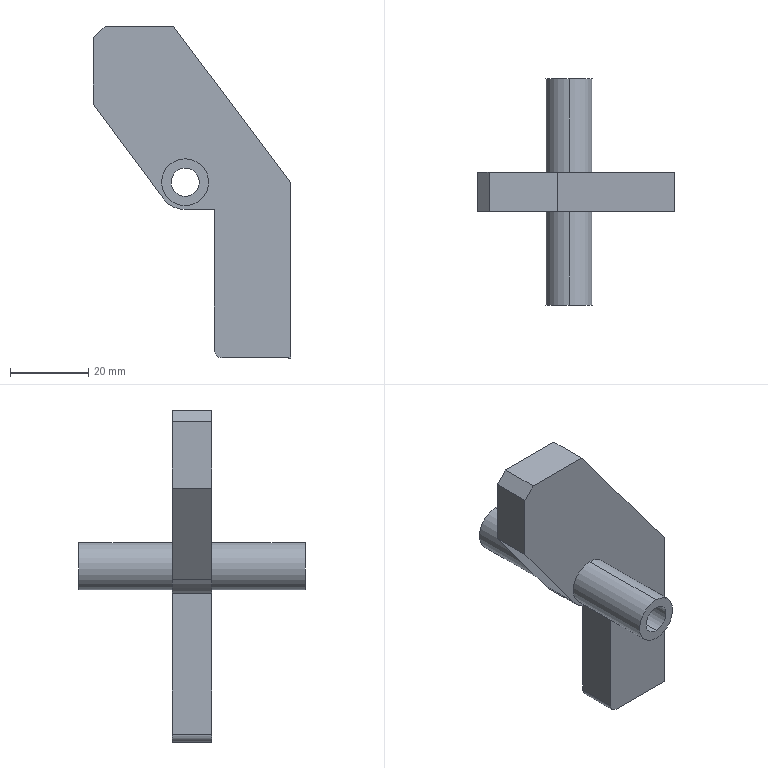Part | SolidWorks | features BaseBody 1 | 1 solid | 21 faces | box 50.5 x 58 x 85 mm | volume 25435 mm3 | plane 13 | cylinder 8 | commonest cylinder face diameters 12 x4 7.2 x2 4 x1 14 x1
STEP:
#1=CARTESIAN_POINT('',(896.946,-3871.973,948.971));
#2=VERTEX_POINT('',#1);
#3=CARTESIAN_POINT('',(896.946,-3871.973,960.971));
#4=VERTEX_POINT('',#3);
#5=CARTESIAN_POINT('',(896.946,-3871.973,954.971));
#6=DIRECTION('',(0.,-1.,0.));
#7=DIRECTION('',(0.,0.,-1.));
#8=AXIS2_PLACEMENT_3D('',#5,#6,#7);
#9=CIRCLE('',#8,6.);
#10=EDGE_CURVE('',#2,#4,#9,.T.);
#11=ORIENTED_EDGE('',*,*,#10,.T.);
#12=CARTESIAN_POINT('',(896.946,-3895.973,960.971));
#13=VERTEX_POINT('',#12);
#14=CARTESIAN_POINT('',(896.946,-3883.973,960.971));
#15=DIRECTION('',(0.,-1.,0.));
#16=VECTOR('',#15,1000.);
#17=LINE('',#14,#16);
#18=EDGE_CURVE('',#4,#13,#17,.T.);
#19=ORIENTED_EDGE('',*,*,#18,.T.);
#20=CARTESIAN_POINT('',(896.946,-3895.973,948.971));
#21=VERTEX_POINT('',#20);
#22=CARTESIAN_POINT('',(896.946,-3895.973,954.971));
#23=DIRECTION('',(0.,-1.,0.));
#24=DIRECTION('',(0.,0.,-1.));
#25=AXIS2_PLACEMENT_3D('',#22,#23,#24);
#26=CIRCLE('',#25,6.);
#27=EDGE_CURVE('',#21,#13,#26,.T.);
#28=ORIENTED_EDGE('',*,*,#27,.F.);
#29=CARTESIAN_POINT('',(896.946,-3883.973,948.971));
#30=DIRECTION('',(0.,-1.,0.));
#31=VECTOR('',#30,1000.);
#32=LINE('',#29,#31);
#33=EDGE_CURVE('',#2,#21,#32,.T.);
#34=ORIENTED_EDGE('',*,*,#33,.F.);
#35=EDGE_LOOP('',(#11,#19,#28,#34));
#36=FACE_OUTER_BOUND('',#35,.T.);
#37=CARTESIAN_POINT('',(896.946,-3883.973,954.971));
#38=DIRECTION('',(0.,-1.,0.));
#39=DIRECTION('',(0.,0.,-1.));
#40=AXIS2_PLACEMENT_3D('',#37,#38,#39);
#41=CYLINDRICAL_SURFACE('',#40,6.);
#42=ADVANCED_FACE('',(#36),#41,.T.);
#43=CARTESIAN_POINT('',(896.946,-3871.973,958.571));
#44=VERTEX_POINT('',#43);
#45=CARTESIAN_POINT('',(896.946,-3871.973,951.371));
#46=VERTEX_POINT('',#45);
#47=CARTESIAN_POINT('',(896.946,-3871.973,954.971));
#48=DIRECTION('',(0.,-1.,0.));
#49=DIRECTION('',(0.,0.,-1.));
#50=AXIS2_PLACEMENT_3D('',#47,#48,#49);
#51=CIRCLE('',#50,3.6);
#52=EDGE_CURVE('',#44,#46,#51,.T.);
#53=ORIENTED_EDGE('',*,*,#52,.F.);
#54=CARTESIAN_POINT('',(896.946,-3929.973,958.571));
#55=VERTEX_POINT('',#54);
#56=CARTESIAN_POINT('',(896.946,-3859.114,958.571));
#57=DIRECTION('',(0.,-1.,0.));
#58=VECTOR('',#57,1000.);
#59=LINE('',#56,#58);
#60=EDGE_CURVE('',#44,#55,#59,.T.);
#61=ORIENTED_EDGE('',*,*,#60,.T.);
#62=CARTESIAN_POINT('',(896.946,-3929.973,951.371));
#63=VERTEX_POINT('',#62);
#64=CARTESIAN_POINT('',(896.946,-3929.973,954.971));
#65=DIRECTION('',(0.,1.,0.));
#66=DIRECTION('',(0.,0.,-1.));
#67=AXIS2_PLACEMENT_3D('',#64,#65,#66);
#68=CIRCLE('',#67,3.6);
#69=EDGE_CURVE('',#63,#55,#68,.T.);
#70=ORIENTED_EDGE('',*,*,#69,.F.);
#71=CARTESIAN_POINT('',(896.946,-3859.114,951.371));
#72=DIRECTION('',(0.,-1.,0.));
#73=VECTOR('',#72,1000.);
#74=LINE('',#71,#73);
#75=EDGE_CURVE('',#46,#63,#74,.T.);
#76=ORIENTED_EDGE('',*,*,#75,.F.);
#77=EDGE_LOOP('',(#53,#61,#70,#76));
#78=FACE_OUTER_BOUND('',#77,.T.);
#79=CARTESIAN_POINT('',(896.946,-3859.114,954.971));
#80=DIRECTION('',(0.,-1.,0.));
#81=DIRECTION('',(0.,0.,-1.));
#82=AXIS2_PLACEMENT_3D('',#79,#80,#81);
#83=CYLINDRICAL_SURFACE('',#82,3.6);
#84=ADVANCED_FACE('',(#78),#83,.F.);
#85=CARTESIAN_POINT('',(896.946,-3905.973,948.971));
#86=VERTEX_POINT('',#85);
#87=CARTESIAN_POINT('',(896.946,-3905.973,960.971));
#88=VERTEX_POINT('',#87);
#89=CARTESIAN_POINT('',(896.946,-3905.973,954.971));
#90=DIRECTION('',(0.,-1.,0.));
#91=DIRECTION('',(0.,0.,-1.));
#92=AXIS2_PLACEMENT_3D('',#89,#90,#91);
#93=CIRCLE('',#92,6.);
#94=EDGE_CURVE('',#86,#88,#93,.T.);
#95=ORIENTED_EDGE('',*,*,#94,.T.);
#96=CARTESIAN_POINT('',(896.946,-3929.973,960.971));
#97=VERTEX_POINT('',#96);
#98=CARTESIAN_POINT('',(896.946,-3917.973,960.971));
#99=DIRECTION('',(0.,-1.,0.));
#100=VECTOR('',#99,1000.);
#101=LINE('',#98,#100);
#102=EDGE_CURVE('',#88,#97,#101,.T.);
#103=ORIENTED_EDGE('',*,*,#102,.T.);
#104=CARTESIAN_POINT('',(896.946,-3929.973,948.971));
#105=VERTEX_POINT('',#104);
#106=CARTESIAN_POINT('',(896.946,-3929.973,954.971));
#107=DIRECTION('',(0.,1.,0.));
#108=DIRECTION('',(0.,0.,-1.));
#109=AXIS2_PLACEMENT_3D('',#106,#107,#108);
#110=CIRCLE('',#109,6.);
#111=EDGE_CURVE('',#97,#105,#110,.T.);
#112=ORIENTED_EDGE('',*,*,#111,.T.);
#113=CARTESIAN_POINT('',(896.946,-3917.973,948.971));
#114=DIRECTION('',(0.,-1.,0.));
#115=VECTOR('',#114,1000.);
#116=LINE('',#113,#115);
#117=EDGE_CURVE('',#86,#105,#116,.T.);
#118=ORIENTED_EDGE('',*,*,#117,.F.);
#119=EDGE_LOOP('',(#95,#103,#112,#118));
#120=FACE_OUTER_BOUND('',#119,.T.);
#121=CARTESIAN_POINT('',(896.946,-3917.973,954.971));
#122=DIRECTION('',(0.,-1.,0.));
#123=DIRECTION('',(0.,0.,-1.));
#124=AXIS2_PLACEMENT_3D('',#121,#122,#123);
#125=CYLINDRICAL_SURFACE('',#124,6.);
#126=ADVANCED_FACE('',(#120),#125,.T.);
#127=ORIENTED_EDGE('',*,*,#27,.T.);
#128=CARTESIAN_POINT('',(896.946,-3895.973,954.971));
#129=DIRECTION('',(0.,-1.,0.));
#130=DIRECTION('',(0.,0.,-1.));
#131=AXIS2_PLACEMENT_3D('',#128,#129,#130);
#132=CIRCLE('',#131,6.);
#133=EDGE_CURVE('',#13,#21,#132,.T.);
#134=ORIENTED_EDGE('',*,*,#133,.T.);
#135=EDGE_LOOP('',(#127,#134));
#136=FACE_BOUND('',#135,.T.);
#137=CARTESIAN_POINT('',(923.946,-3895.973,954.971));
#138=VERTEX_POINT('',#137);
#139=CARTESIAN_POINT('',(923.946,-3895.973,909.971));
#140=VERTEX_POINT('',#139);
#141=CARTESIAN_POINT('',(923.946,-3895.973,957.966));
#142=DIRECTION('',(0.,0.,-1.));
#143=VECTOR('',#142,1000.);
#144=LINE('',#141,#143);
#145=EDGE_CURVE('',#138,#140,#144,.T.);
#146=ORIENTED_EDGE('',*,*,#145,.T.);
#147=CARTESIAN_POINT('',(906.446,-3895.973,909.971));
#148=VERTEX_POINT('',#147);
#149=CARTESIAN_POINT('',(901.414,-3895.973,909.971));
#150=DIRECTION('',(-1.,0.,0.));
#151=VECTOR('',#150,1000.);
#152=LINE('',#149,#151);
#153=EDGE_CURVE('',#140,#148,#152,.T.);
#154=ORIENTED_EDGE('',*,*,#153,.T.);
#155=CARTESIAN_POINT('',(904.446,-3895.973,911.971));
#156=VERTEX_POINT('',#155);
#157=CARTESIAN_POINT('',(906.446,-3895.973,911.971));
#158=DIRECTION('',(0.,1.,0.));
#159=DIRECTION('',(0.,0.,-1.));
#160=AXIS2_PLACEMENT_3D('',#157,#158,#159);
#161=CIRCLE('',#160,2.);
#162=EDGE_CURVE('',#148,#156,#161,.T.);
#163=ORIENTED_EDGE('',*,*,#162,.T.);
#164=CARTESIAN_POINT('',(904.446,-3895.973,947.971));
#165=VERTEX_POINT('',#164);
#166=CARTESIAN_POINT('',(904.446,-3895.973,957.966));
#167=DIRECTION('',(0.,0.,1.));
#168=VECTOR('',#167,1000.);
#169=LINE('',#166,#168);
#170=EDGE_CURVE('',#156,#165,#169,.T.);
#171=ORIENTED_EDGE('',*,*,#170,.T.);
#172=CARTESIAN_POINT('',(896.946,-3895.973,947.971));
#173=VERTEX_POINT('',#172);
#174=CARTESIAN_POINT('',(901.414,-3895.973,947.971));
#175=DIRECTION('',(-1.,0.,0.));
#176=VECTOR('',#175,1000.);
#177=LINE('',#174,#176);
#178=EDGE_CURVE('',#165,#173,#177,.T.);
#179=ORIENTED_EDGE('',*,*,#178,.T.);
#180=CARTESIAN_POINT('',(890.807,-3895.973,951.607));
#181=VERTEX_POINT('',#180);
#182=CARTESIAN_POINT('',(896.946,-3895.973,954.971));
#183=DIRECTION('',(0.,1.,0.));
#184=DIRECTION('',(0.,0.,-1.));
#185=AXIS2_PLACEMENT_3D('',#182,#183,#184);
#186=CIRCLE('',#185,7.);
#187=EDGE_CURVE('',#173,#181,#186,.T.);
#188=ORIENTED_EDGE('',*,*,#187,.T.);
#189=CARTESIAN_POINT('',(873.446,-3895.973,974.971));
#190=VERTEX_POINT('',#189);
#191=CARTESIAN_POINT('',(890.807,-3895.973,951.607));
#192=DIRECTION('',(-0.5964,0.,0.8027));
#193=VECTOR('',#192,1000.);
#194=LINE('',#191,#193);
#195=EDGE_CURVE('',#181,#190,#194,.T.);
#196=ORIENTED_EDGE('',*,*,#195,.T.);
#197=CARTESIAN_POINT('',(873.446,-3895.973,991.971));
#198=VERTEX_POINT('',#197);
#199=CARTESIAN_POINT('',(873.446,-3895.973,957.966));
#200=DIRECTION('',(0.,0.,1.));
#201=VECTOR('',#200,1000.);
#202=LINE('',#199,#201);
#203=EDGE_CURVE('',#190,#198,#202,.T.);
#204=ORIENTED_EDGE('',*,*,#203,.T.);
#205=CARTESIAN_POINT('',(876.446,-3895.973,994.971));
#206=VERTEX_POINT('',#205);
#207=CARTESIAN_POINT('',(873.446,-3895.973,991.971));
#208=DIRECTION('',(0.7071,0.,0.7071));
#209=VECTOR('',#208,1000.);
#210=LINE('',#207,#209);
#211=EDGE_CURVE('',#198,#206,#210,.T.);
#212=ORIENTED_EDGE('',*,*,#211,.T.);
#213=CARTESIAN_POINT('',(893.946,-3895.973,994.971));
#214=VERTEX_POINT('',#213);
#215=CARTESIAN_POINT('',(901.414,-3895.973,994.971));
#216=DIRECTION('',(1.,0.,0.));
#217=VECTOR('',#216,1000.);
#218=LINE('',#215,#217);
#219=EDGE_CURVE('',#206,#214,#218,.T.);
#220=ORIENTED_EDGE('',*,*,#219,.T.);
#221=CARTESIAN_POINT('',(893.946,-3895.973,994.971));
#222=DIRECTION('',(0.6,0.,-0.8));
#223=VECTOR('',#222,1000.);
#224=LINE('',#221,#223);
#225=EDGE_CURVE('',#214,#138,#224,.T.);
#226=ORIENTED_EDGE('',*,*,#225,.T.);
#227=EDGE_LOOP('',(#146,#154,#163,#171,#179,#188,#196,#204,#212,#220,#226));
#228=FACE_OUTER_BOUND('',#227,.T.);
#229=CARTESIAN_POINT('',(901.414,-3895.973,957.966));
#230=DIRECTION('',(0.,1.,0.));
#231=DIRECTION('',(0.,0.,1.));
#232=AXIS2_PLACEMENT_3D('',#229,#230,#231);
#233=PLANE('',#232);
#234=ADVANCED_FACE('',(#136,#228),#233,.T.);
#235=ORIENTED_EDGE('',*,*,#18,.F.);
#236=CARTESIAN_POINT('',(896.946,-3871.973,954.971));
#237=DIRECTION('',(0.,-1.,0.));
#238=DIRECTION('',(0.,0.,-1.));
#239=AXIS2_PLACEMENT_3D('',#236,#237,#238);
#240=CIRCLE('',#239,6.);
#241=EDGE_CURVE('',#4,#2,#240,.T.);
#242=ORIENTED_EDGE('',*,*,#241,.T.);
#243=ORIENTED_EDGE('',*,*,#33,.T.);
#244=ORIENTED_EDGE('',*,*,#133,.F.);
#245=EDGE_LOOP('',(#235,#242,#243,#244));
#246=FACE_OUTER_BOUND('',#245,.T.);
#247=CARTESIAN_POINT('',(896.946,-3883.973,954.971));
#248=DIRECTION('',(0.,-1.,0.));
#249=DIRECTION('',(0.,0.,-1.));
#250=AXIS2_PLACEMENT_3D('',#247,#248,#249);
#251=CYLINDRICAL_SURFACE('',#250,6.);
#252=ADVANCED_FACE('',(#246),#251,.T.);
#253=ORIENTED_EDGE('',*,*,#153,.F.);
#254=CARTESIAN_POINT('',(923.946,-3905.973,909.971));
#255=VERTEX_POINT('',#254);
#256=CARTESIAN_POINT('',(923.946,-3895.973,909.971));
#257=DIRECTION('',(0.,-1.,0.));
#258=VECTOR('',#257,1000.);
#259=LINE('',#256,#258);
#260=EDGE_CURVE('',#140,#255,#259,.T.);
#261=ORIENTED_EDGE('',*,*,#260,.T.);
#262=CARTESIAN_POINT('',(906.446,-3905.973,909.971));
#263=VERTEX_POINT('',#262);
#264=CARTESIAN_POINT('',(923.946,-3905.973,909.971));
#265=DIRECTION('',(-1.,0.,0.));
#266=VECTOR('',#265,1000.);
#267=LINE('',#264,#266);
#268=EDGE_CURVE('',#255,#263,#267,.T.);
#269=ORIENTED_EDGE('',*,*,#268,.T.);
#270=CARTESIAN_POINT('',(906.446,-3895.973,909.971));
#271=DIRECTION('',(0.,1.,0.));
#272=VECTOR('',#271,1000.);
#273=LINE('',#270,#272);
#274=EDGE_CURVE('',#263,#148,#273,.T.);
#275=ORIENTED_EDGE('',*,*,#274,.T.);
#276=EDGE_LOOP('',(#253,#261,#269,#275));
#277=FACE_OUTER_BOUND('',#276,.T.);
#278=CARTESIAN_POINT('',(923.946,-3895.973,909.971));
#279=DIRECTION('',(0.,0.,-1.));
#280=DIRECTION('',(-1.,0.,0.));
#281=AXIS2_PLACEMENT_3D('',#278,#279,#280);
#282=PLANE('',#281);
#283=ADVANCED_FACE('',(#277),#282,.T.);
#284=ORIENTED_EDGE('',*,*,#145,.F.);
#285=CARTESIAN_POINT('',(923.946,-3905.973,954.971));
#286=VERTEX_POINT('',#285);
#287=CARTESIAN_POINT('',(923.946,-3895.973,954.971));
#288=DIRECTION('',(0.,-1.,0.));
#289=VECTOR('',#288,1000.);
#290=LINE('',#287,#289);
#291=EDGE_CURVE('',#138,#286,#290,.T.);
#292=ORIENTED_EDGE('',*,*,#291,.T.);
#293=CARTESIAN_POINT('',(923.946,-3905.973,954.971));
#294=DIRECTION('',(0.,0.,-1.));
#295=VECTOR('',#294,1000.);
#296=LINE('',#293,#295);
#297=EDGE_CURVE('',#286,#255,#296,.T.);
#298=ORIENTED_EDGE('',*,*,#297,.T.);
#299=ORIENTED_EDGE('',*,*,#260,.F.);
#300=EDGE_LOOP('',(#284,#292,#298,#299));
#301=FACE_OUTER_BOUND('',#300,.T.);
#302=CARTESIAN_POINT('',(923.946,-3895.973,954.971));
#303=DIRECTION('',(1.,0.,0.));
#304=DIRECTION('',(0.,0.,-1.));
#305=AXIS2_PLACEMENT_3D('',#302,#303,#304);
#306=PLANE('',#305);
#307=ADVANCED_FACE('',(#301),#306,.T.);
#308=ORIENTED_EDGE('',*,*,#225,.F.);
#309=CARTESIAN_POINT('',(893.946,-3905.973,994.971));
#310=VERTEX_POINT('',#309);
#311=CARTESIAN_POINT('',(893.946,-3895.973,994.971));
#312=DIRECTION('',(0.,-1.,0.));
#313=VECTOR('',#312,1000.);
#314=LINE('',#311,#313);
#315=EDGE_CURVE('',#214,#310,#314,.T.);
#316=ORIENTED_EDGE('',*,*,#315,.T.);
#317=CARTESIAN_POINT('',(893.946,-3905.973,994.971));
#318=DIRECTION('',(0.6,0.,-0.8));
#319=VECTOR('',#318,1000.);
#320=LINE('',#317,#319);
#321=EDGE_CURVE('',#310,#286,#320,.T.);
#322=ORIENTED_EDGE('',*,*,#321,.T.);
#323=ORIENTED_EDGE('',*,*,#291,.F.);
#324=EDGE_LOOP('',(#308,#316,#322,#323));
#325=FACE_OUTER_BOUND('',#324,.T.);
#326=CARTESIAN_POINT('',(893.946,-3895.973,994.971));
#327=DIRECTION('',(0.8,0.,0.6));
#328=DIRECTION('',(0.6,0.,-0.8));
#329=AXIS2_PLACEMENT_3D('',#326,#327,#328);
#330=PLANE('',#329);
#331=ADVANCED_FACE('',(#325),#330,.T.);
#332=ORIENTED_EDGE('',*,*,#219,.F.);
#333=CARTESIAN_POINT('',(876.446,-3905.973,994.971));
#334=VERTEX_POINT('',#333);
#335=CARTESIAN_POINT('',(876.446,-3895.973,994.971));
#336=DIRECTION('',(0.,-1.,0.));
#337=VECTOR('',#336,1000.);
#338=LINE('',#335,#337);
#339=EDGE_CURVE('',#206,#334,#338,.T.);
#340=ORIENTED_EDGE('',*,*,#339,.T.);
#341=CARTESIAN_POINT('',(876.446,-3905.973,994.971));
#342=DIRECTION('',(1.,0.,0.));
#343=VECTOR('',#342,1000.);
#344=LINE('',#341,#343);
#345=EDGE_CURVE('',#334,#310,#344,.T.);
#346=ORIENTED_EDGE('',*,*,#345,.T.);
#347=ORIENTED_EDGE('',*,*,#315,.F.);
#348=EDGE_LOOP('',(#332,#340,#346,#347));
#349=FACE_OUTER_BOUND('',#348,.T.);
#350=CARTESIAN_POINT('',(876.446,-3895.973,994.971));
#351=DIRECTION('',(0.,0.,1.));
#352=DIRECTION('',(1.,0.,0.));
#353=AXIS2_PLACEMENT_3D('',#350,#351,#352);
#354=PLANE('',#353);
#355=ADVANCED_FACE('',(#349),#354,.T.);
#356=ORIENTED_EDGE('',*,*,#211,.F.);
#357=CARTESIAN_POINT('',(873.446,-3905.973,991.971));
#358=VERTEX_POINT('',#357);
#359=CARTESIAN_POINT('',(873.446,-3895.973,991.971));
#360=DIRECTION('',(0.,-1.,0.));
#361=VECTOR('',#360,1000.);
#362=LINE('',#359,#361);
#363=EDGE_CURVE('',#198,#358,#362,.T.);
#364=ORIENTED_EDGE('',*,*,#363,.T.);
#365=CARTESIAN_POINT('',(873.446,-3905.973,991.971));
#366=DIRECTION('',(0.7071,0.,0.7071));
#367=VECTOR('',#366,1000.);
#368=LINE('',#365,#367);
#369=EDGE_CURVE('',#358,#334,#368,.T.);
#370=ORIENTED_EDGE('',*,*,#369,.T.);
#371=ORIENTED_EDGE('',*,*,#339,.F.);
#372=EDGE_LOOP('',(#356,#364,#370,#371));
#373=FACE_OUTER_BOUND('',#372,.T.);
#374=CARTESIAN_POINT('',(873.446,-3895.973,991.971));
#375=DIRECTION('',(-0.7071,0.,0.7071));
#376=DIRECTION('',(0.7071,0.,0.7071));
#377=AXIS2_PLACEMENT_3D('',#374,#375,#376);
#378=PLANE('',#377);
#379=ADVANCED_FACE('',(#373),#378,.T.);
#380=ORIENTED_EDGE('',*,*,#203,.F.);
#381=CARTESIAN_POINT('',(873.446,-3905.973,974.971));
#382=VERTEX_POINT('',#381);
#383=CARTESIAN_POINT('',(873.446,-3895.973,974.971));
#384=DIRECTION('',(0.,-1.,0.));
#385=VECTOR('',#384,1000.);
#386=LINE('',#383,#385);
#387=EDGE_CURVE('',#190,#382,#386,.T.);
#388=ORIENTED_EDGE('',*,*,#387,.T.);
#389=CARTESIAN_POINT('',(873.446,-3905.973,974.971));
#390=DIRECTION('',(0.,0.,1.));
#391=VECTOR('',#390,1000.);
#392=LINE('',#389,#391);
#393=EDGE_CURVE('',#382,#358,#392,.T.);
#394=ORIENTED_EDGE('',*,*,#393,.T.);
#395=ORIENTED_EDGE('',*,*,#363,.F.);
#396=EDGE_LOOP('',(#380,#388,#394,#395));
#397=FACE_OUTER_BOUND('',#396,.T.);
#398=CARTESIAN_POINT('',(873.446,-3895.973,974.971));
#399=DIRECTION('',(-1.,0.,0.));
#400=DIRECTION('',(0.,0.,1.));
#401=AXIS2_PLACEMENT_3D('',#398,#399,#400);
#402=PLANE('',#401);
#403=ADVANCED_FACE('',(#397),#402,.T.);
#404=ORIENTED_EDGE('',*,*,#195,.F.);
#405=CARTESIAN_POINT('',(890.807,-3905.973,951.607));
#406=VERTEX_POINT('',#405);
#407=CARTESIAN_POINT('',(890.807,-3895.973,951.607));
#408=DIRECTION('',(0.,-1.,0.));
#409=VECTOR('',#408,1000.);
#410=LINE('',#407,#409);
#411=EDGE_CURVE('',#181,#406,#410,.T.);
#412=ORIENTED_EDGE('',*,*,#411,.T.);
#413=CARTESIAN_POINT('',(890.807,-3905.973,951.607));
#414=DIRECTION('',(-0.5964,0.,0.8027));
#415=VECTOR('',#414,1000.);
#416=LINE('',#413,#415);
#417=EDGE_CURVE('',#406,#382,#416,.T.);
#418=ORIENTED_EDGE('',*,*,#417,.T.);
#419=ORIENTED_EDGE('',*,*,#387,.F.);
#420=EDGE_LOOP('',(#404,#412,#418,#419));
#421=FACE_OUTER_BOUND('',#420,.T.);
#422=CARTESIAN_POINT('',(890.807,-3895.973,951.607));
#423=DIRECTION('',(-0.8027,0.,-0.5964));
#424=DIRECTION('',(-0.5964,0.,0.8027));
#425=AXIS2_PLACEMENT_3D('',#422,#423,#424);
#426=PLANE('',#425);
#427=ADVANCED_FACE('',(#421),#426,.T.);
#428=ORIENTED_EDGE('',*,*,#187,.F.);
#429=CARTESIAN_POINT('',(896.946,-3905.973,947.971));
#430=VERTEX_POINT('',#429);
#431=CARTESIAN_POINT('',(896.946,-3895.973,947.971));
#432=DIRECTION('',(0.,-1.,0.));
#433=VECTOR('',#432,1000.);
#434=LINE('',#431,#433);
#435=EDGE_CURVE('',#173,#430,#434,.T.);
#436=ORIENTED_EDGE('',*,*,#435,.T.);
#437=CARTESIAN_POINT('',(896.946,-3905.973,954.971));
#438=DIRECTION('',(0.,1.,0.));
#439=DIRECTION('',(0.,0.,-1.));
#440=AXIS2_PLACEMENT_3D('',#437,#438,#439);
#441=CIRCLE('',#440,7.);
#442=EDGE_CURVE('',#430,#406,#441,.T.);
#443=ORIENTED_EDGE('',*,*,#442,.T.);
#444=ORIENTED_EDGE('',*,*,#411,.F.);
#445=EDGE_LOOP('',(#428,#436,#443,#444));
#446=FACE_OUTER_BOUND('',#445,.T.);
#447=CARTESIAN_POINT('',(896.946,-3895.973,954.971));
#448=DIRECTION('',(0.,-1.,0.));
#449=DIRECTION('',(0.,0.,-1.));
#450=AXIS2_PLACEMENT_3D('',#447,#448,#449);
#451=CYLINDRICAL_SURFACE('',#450,7.);
#452=ADVANCED_FACE('',(#446),#451,.T.);
#453=ORIENTED_EDGE('',*,*,#178,.F.);
#454=CARTESIAN_POINT('',(904.446,-3905.973,947.971));
#455=VERTEX_POINT('',#454);
#456=CARTESIAN_POINT('',(904.446,-3895.973,947.971));
#457=DIRECTION('',(0.,-1.,0.));
#458=VECTOR('',#457,1000.);
#459=LINE('',#456,#458);
#460=EDGE_CURVE('',#165,#455,#459,.T.);
#461=ORIENTED_EDGE('',*,*,#460,.T.);
#462=CARTESIAN_POINT('',(904.446,-3905.973,947.971));
#463=DIRECTION('',(-1.,0.,0.));
#464=VECTOR('',#463,1000.);
#465=LINE('',#462,#464);
#466=EDGE_CURVE('',#455,#430,#465,.T.);
#467=ORIENTED_EDGE('',*,*,#466,.T.);
#468=ORIENTED_EDGE('',*,*,#435,.F.);
#469=EDGE_LOOP('',(#453,#461,#467,#468));
#470=FACE_OUTER_BOUND('',#469,.T.);
#471=CARTESIAN_POINT('',(904.446,-3895.973,947.971));
#472=DIRECTION('',(0.,0.,-1.));
#473=DIRECTION('',(-1.,0.,0.));
#474=AXIS2_PLACEMENT_3D('',#471,#472,#473);
#475=PLANE('',#474);
#476=ADVANCED_FACE('',(#470),#475,.T.);
#477=ORIENTED_EDGE('',*,*,#170,.F.);
#478=CARTESIAN_POINT('',(904.446,-3905.973,911.971));
#479=VERTEX_POINT('',#478);
#480=CARTESIAN_POINT('',(904.446,-3895.973,911.971));
#481=DIRECTION('',(0.,-1.,0.));
#482=VECTOR('',#481,1000.);
#483=LINE('',#480,#482);
#484=EDGE_CURVE('',#156,#479,#483,.T.);
#485=ORIENTED_EDGE('',*,*,#484,.T.);
#486=CARTESIAN_POINT('',(904.446,-3905.973,911.971));
#487=DIRECTION('',(0.,0.,1.));
#488=VECTOR('',#487,1000.);
#489=LINE('',#486,#488);
#490=EDGE_CURVE('',#479,#455,#489,.T.);
#491=ORIENTED_EDGE('',*,*,#490,.T.);
#492=ORIENTED_EDGE('',*,*,#460,.F.);
#493=EDGE_LOOP('',(#477,#485,#491,#492));
#494=FACE_OUTER_BOUND('',#493,.T.);
#495=CARTESIAN_POINT('',(904.446,-3895.973,911.971));
#496=DIRECTION('',(-1.,0.,0.));
#497=DIRECTION('',(0.,0.,1.));
#498=AXIS2_PLACEMENT_3D('',#495,#496,#497);
#499=PLANE('',#498);
#500=ADVANCED_FACE('',(#494),#499,.T.);
#501=ORIENTED_EDGE('',*,*,#162,.F.);
#502=ORIENTED_EDGE('',*,*,#274,.F.);
#503=CARTESIAN_POINT('',(906.446,-3905.973,911.971));
#504=DIRECTION('',(0.,1.,0.));
#505=DIRECTION('',(0.,0.,-1.));
#506=AXIS2_PLACEMENT_3D('',#503,#504,#505);
#507=CIRCLE('',#506,2.);
#508=EDGE_CURVE('',#263,#479,#507,.T.);
#509=ORIENTED_EDGE('',*,*,#508,.T.);
#510=ORIENTED_EDGE('',*,*,#484,.F.);
#511=EDGE_LOOP('',(#501,#502,#509,#510));
#512=FACE_OUTER_BOUND('',#511,.T.);
#513=CARTESIAN_POINT('',(906.446,-3895.973,911.971));
#514=DIRECTION('',(0.,-1.,0.));
#515=DIRECTION('',(0.,0.,-1.));
#516=AXIS2_PLACEMENT_3D('',#513,#514,#515);
#517=CYLINDRICAL_SURFACE('',#516,2.);
#518=ADVANCED_FACE('',(#512),#517,.T.);
#519=ORIENTED_EDGE('',*,*,#10,.F.);
#520=ORIENTED_EDGE('',*,*,#241,.F.);
#521=EDGE_LOOP('',(#519,#520));
#522=FACE_OUTER_BOUND('',#521,.T.);
#523=CARTESIAN_POINT('',(896.946,-3871.973,954.971));
#524=DIRECTION('',(0.,-1.,0.));
#525=DIRECTION('',(0.,0.,-1.));
#526=AXIS2_PLACEMENT_3D('',#523,#524,#525);
#527=CIRCLE('',#526,3.6);
#528=EDGE_CURVE('',#46,#44,#527,.T.);
#529=ORIENTED_EDGE('',*,*,#528,.T.);
#530=ORIENTED_EDGE('',*,*,#52,.T.);
#531=EDGE_LOOP('',(#529,#530));
#532=FACE_BOUND('',#531,.T.);
#533=CARTESIAN_POINT('',(896.946,-3871.973,954.971));
#534=DIRECTION('',(0.,1.,0.));
#535=DIRECTION('',(0.,0.,1.));
#536=AXIS2_PLACEMENT_3D('',#533,#534,#535);
#537=PLANE('',#536);
#538=ADVANCED_FACE('',(#522,#532),#537,.T.);
#539=ORIENTED_EDGE('',*,*,#508,.F.);
#540=ORIENTED_EDGE('',*,*,#268,.F.);
#541=ORIENTED_EDGE('',*,*,#297,.F.);
#542=ORIENTED_EDGE('',*,*,#321,.F.);
#543=ORIENTED_EDGE('',*,*,#345,.F.);
#544=ORIENTED_EDGE('',*,*,#369,.F.);
#545=ORIENTED_EDGE('',*,*,#393,.F.);
#546=ORIENTED_EDGE('',*,*,#417,.F.);
#547=ORIENTED_EDGE('',*,*,#442,.F.);
#548=ORIENTED_EDGE('',*,*,#466,.F.);
#549=ORIENTED_EDGE('',*,*,#490,.F.);
#550=EDGE_LOOP('',(#539,#540,#541,#542,#543,#544,#545,#546,#547,#548,#549));
#551=FACE_OUTER_BOUND('',#550,.T.);
#552=ORIENTED_EDGE('',*,*,#94,.F.);
#553=CARTESIAN_POINT('',(896.946,-3905.973,954.971));
#554=DIRECTION('',(0.,-1.,0.));
#555=DIRECTION('',(0.,0.,-1.));
#556=AXIS2_PLACEMENT_3D('',#553,#554,#555);
#557=CIRCLE('',#556,6.);
#558=EDGE_CURVE('',#88,#86,#557,.T.);
#559=ORIENTED_EDGE('',*,*,#558,.F.);
#560=EDGE_LOOP('',(#552,#559));
#561=FACE_BOUND('',#560,.T.);
#562=CARTESIAN_POINT('',(901.414,-3905.973,957.966));
#563=DIRECTION('',(0.,1.,0.));
#564=DIRECTION('',(0.,0.,1.));
#565=AXIS2_PLACEMENT_3D('',#562,#563,#564);
#566=PLANE('',#565);
#567=ADVANCED_FACE('',(#551,#561),#566,.F.);
#568=ORIENTED_EDGE('',*,*,#60,.F.);
#569=ORIENTED_EDGE('',*,*,#528,.F.);
#570=ORIENTED_EDGE('',*,*,#75,.T.);
#571=CARTESIAN_POINT('',(896.946,-3929.973,954.971));
#572=DIRECTION('',(0.,1.,0.));
#573=DIRECTION('',(0.,0.,-1.));
#574=AXIS2_PLACEMENT_3D('',#571,#572,#573);
#575=CIRCLE('',#574,3.6);
#576=EDGE_CURVE('',#55,#63,#575,.T.);
#577=ORIENTED_EDGE('',*,*,#576,.F.);
#578=EDGE_LOOP('',(#568,#569,#570,#577));
#579=FACE_OUTER_BOUND('',#578,.T.);
#580=CARTESIAN_POINT('',(896.946,-3859.114,954.971));
#581=DIRECTION('',(0.,-1.,0.));
#582=DIRECTION('',(0.,0.,-1.));
#583=AXIS2_PLACEMENT_3D('',#580,#581,#582);
#584=CYLINDRICAL_SURFACE('',#583,3.6);
#585=ADVANCED_FACE('',(#579),#584,.F.);
#586=ORIENTED_EDGE('',*,*,#102,.F.);
#587=ORIENTED_EDGE('',*,*,#558,.T.);
#588=ORIENTED_EDGE('',*,*,#117,.T.);
#589=CARTESIAN_POINT('',(896.946,-3929.973,954.971));
#590=DIRECTION('',(0.,1.,0.));
#591=DIRECTION('',(0.,0.,-1.));
#592=AXIS2_PLACEMENT_3D('',#589,#590,#591);
#593=CIRCLE('',#592,6.);
#594=EDGE_CURVE('',#105,#97,#593,.T.);
#595=ORIENTED_EDGE('',*,*,#594,.T.);
#596=EDGE_LOOP('',(#586,#587,#588,#595));
#597=FACE_OUTER_BOUND('',#596,.T.);
#598=CARTESIAN_POINT('',(896.946,-3917.973,954.971));
#599=DIRECTION('',(0.,-1.,0.));
#600=DIRECTION('',(0.,0.,-1.));
#601=AXIS2_PLACEMENT_3D('',#598,#599,#600);
#602=CYLINDRICAL_SURFACE('',#601,6.);
#603=ADVANCED_FACE('',(#597),#602,.T.);
#604=ORIENTED_EDGE('',*,*,#594,.F.);
#605=ORIENTED_EDGE('',*,*,#111,.F.);
#606=EDGE_LOOP('',(#604,#605));
#607=FACE_OUTER_BOUND('',#606,.T.);
#608=ORIENTED_EDGE('',*,*,#69,.T.);
#609=ORIENTED_EDGE('',*,*,#576,.T.);
#610=EDGE_LOOP('',(#608,#609));
#611=FACE_BOUND('',#610,.T.);
#612=CARTESIAN_POINT('',(896.946,-3929.973,954.971));
#613=DIRECTION('',(0.,-1.,0.));
#614=DIRECTION('',(0.,0.,-1.));
#615=AXIS2_PLACEMENT_3D('',#612,#613,#614);
#616=PLANE('',#615);
#617=ADVANCED_FACE('',(#607,#611),#616,.T.);
#618=CLOSED_SHELL('',(#42,#84,#126,#234,#252,#283,#307,#331,#355,#379,#403,#427,#452,#476,#500,#518,#538,#567,#585,#603,#617));
#619=MANIFOLD_SOLID_BREP('',#618);
#620=CARTESIAN_POINT('',(0.,0.,0.));
#621=DIRECTION('',(0.,0.,1.));
#622=DIRECTION('',(1.,0.,0.));
#623=AXIS2_PLACEMENT_3D('',#620,#621,#622);
#624=(LENGTH_UNIT()NAMED_UNIT(*)SI_UNIT(.MILLI.,.METRE.));
#625=UNCERTAINTY_MEASURE_WITH_UNIT(LENGTH_MEASURE(0.00001),#624,'','');
#626=(NAMED_UNIT(*)PLANE_ANGLE_UNIT()SI_UNIT($,.RADIAN.));
#627=(NAMED_UNIT(*)SI_UNIT($,.STERADIAN.)SOLID_ANGLE_UNIT());
#628=(GEOMETRIC_REPRESENTATION_CONTEXT(3)GLOBAL_UNCERTAINTY_ASSIGNED_CONTEXT((#625))GLOBAL_UNIT_ASSIGNED_CONTEXT((#624,#626,#627))REPRESENTATION_CONTEXT('',''));
#629=ADVANCED_BREP_SHAPE_REPRESENTATION('',(#619,#623),#628);